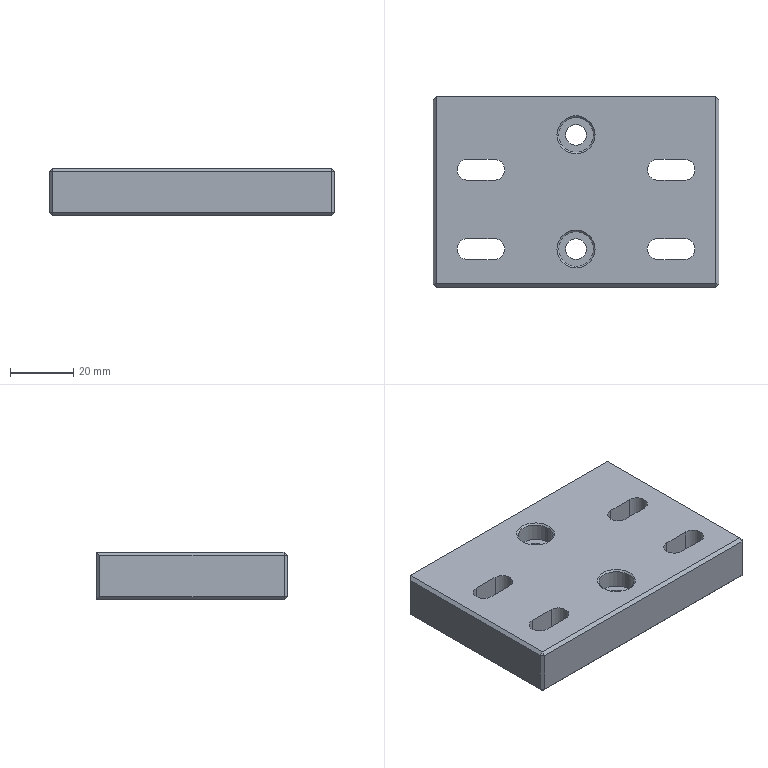Part | SolidWorks | features HoleWzd 3, Chamfer 1, Extrusion 1 | 1 solid | 110 faces | box 90 x 60 x 15 mm | volume 70630 mm3 | plane 50 | cylinder 36 | cone 24 | commonest cylinder face diameters 6.6 x16 11 x16 5 x4